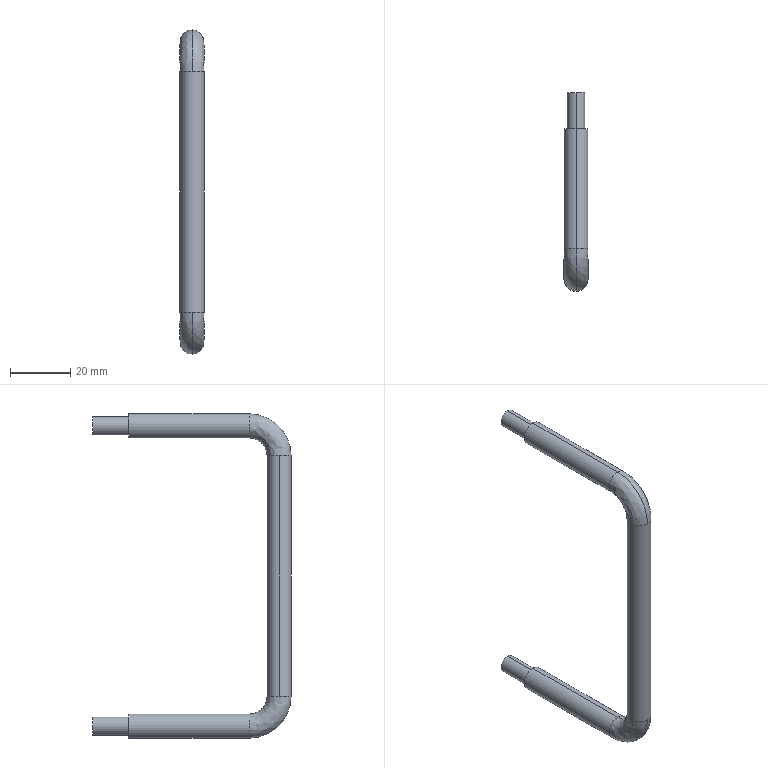Part | SolidWorks | features BaseBody 1 | 1 solid | 18 faces | box 8 x 66 x 108 mm | volume 10300 mm3 | cylinder 10 | spline 4 | plane 4 | commonest cylinder face diameters 8 x6 6 x4
STEP:
#1=CARTESIAN_POINT('',(331.946,-4131.973,2124.971));
#2=VERTEX_POINT('',#1);
#3=CARTESIAN_POINT('',(335.946,-4135.973,2124.971));
#4=VERTEX_POINT('',#3);
#5=CARTESIAN_POINT('',(331.946,-4135.973,2124.971));
#6=DIRECTION('',(0.,0.,-1.));
#7=DIRECTION('',(-1.,0.,0.));
#8=AXIS2_PLACEMENT_3D('',#5,#6,#7);
#9=CIRCLE('',#8,4.);
#10=EDGE_CURVE('',#2,#4,#9,.T.);
#11=ORIENTED_EDGE('',*,*,#10,.T.);
#12=CARTESIAN_POINT('',(335.946,-4135.973,2044.971));
#13=VERTEX_POINT('',#12);
#14=CARTESIAN_POINT('',(335.946,-4135.973,2044.971));
#15=DIRECTION('',(0.,0.,-1.));
#16=VECTOR('',#15,1000.);
#17=LINE('',#14,#16);
#18=EDGE_CURVE('',#4,#13,#17,.T.);
#19=ORIENTED_EDGE('',*,*,#18,.T.);
#20=CARTESIAN_POINT('',(331.946,-4131.973,2044.971));
#21=VERTEX_POINT('',#20);
#22=CARTESIAN_POINT('',(331.946,-4135.973,2044.971));
#23=DIRECTION('',(0.,0.,1.));
#24=DIRECTION('',(-1.,0.,0.));
#25=AXIS2_PLACEMENT_3D('',#22,#23,#24);
#26=CIRCLE('',#25,4.);
#27=EDGE_CURVE('',#13,#21,#26,.T.);
#28=ORIENTED_EDGE('',*,*,#27,.T.);
#29=CARTESIAN_POINT('',(327.946,-4135.973,2044.971));
#30=VERTEX_POINT('',#29);
#31=CARTESIAN_POINT('',(331.946,-4135.973,2044.971));
#32=DIRECTION('',(0.,0.,1.));
#33=DIRECTION('',(-1.,0.,0.));
#34=AXIS2_PLACEMENT_3D('',#31,#32,#33);
#35=CIRCLE('',#34,4.);
#36=EDGE_CURVE('',#21,#30,#35,.T.);
#37=ORIENTED_EDGE('',*,*,#36,.T.);
#38=CARTESIAN_POINT('',(327.946,-4135.973,2124.971));
#39=VERTEX_POINT('',#38);
#40=CARTESIAN_POINT('',(327.946,-4135.973,2044.971));
#41=DIRECTION('',(0.,0.,-1.));
#42=VECTOR('',#41,1000.);
#43=LINE('',#40,#42);
#44=EDGE_CURVE('',#39,#30,#43,.T.);
#45=ORIENTED_EDGE('',*,*,#44,.F.);
#46=CARTESIAN_POINT('',(331.946,-4135.973,2124.971));
#47=DIRECTION('',(0.,0.,-1.));
#48=DIRECTION('',(-1.,0.,0.));
#49=AXIS2_PLACEMENT_3D('',#46,#47,#48);
#50=CIRCLE('',#49,4.);
#51=EDGE_CURVE('',#39,#2,#50,.T.);
#52=ORIENTED_EDGE('',*,*,#51,.T.);
#53=EDGE_LOOP('',(#11,#19,#28,#37,#45,#52));
#54=FACE_OUTER_BOUND('',#53,.T.);
#55=CARTESIAN_POINT('',(331.946,-4135.973,2044.971));
#56=DIRECTION('',(0.,0.,-1.));
#57=DIRECTION('',(-1.,0.,0.));
#58=AXIS2_PLACEMENT_3D('',#55,#56,#57);
#59=CYLINDRICAL_SURFACE('',#58,4.);
#60=ADVANCED_FACE('',(#54),#59,.T.);
#61=ORIENTED_EDGE('',*,*,#36,.F.);
#62=CARTESIAN_POINT('',(331.946,-4125.973,2038.971));
#63=VERTEX_POINT('',#62);
#64=CARTESIAN_POINT('',(331.946,-4125.973,2044.971));
#65=DIRECTION('',(1.,0.,0.));
#66=DIRECTION('',(0.,0.,1.));
#67=AXIS2_PLACEMENT_3D('',#64,#65,#66);
#68=CIRCLE('',#67,6.);
#69=EDGE_CURVE('',#21,#63,#68,.T.);
#70=ORIENTED_EDGE('',*,*,#69,.T.);
#71=CARTESIAN_POINT('',(331.946,-4125.973,2030.971));
#72=VERTEX_POINT('',#71);
#73=CARTESIAN_POINT('',(331.946,-4125.973,2034.971));
#74=DIRECTION('',(0.,-1.,0.));
#75=DIRECTION('',(0.,0.,-1.));
#76=AXIS2_PLACEMENT_3D('',#73,#74,#75);
#77=CIRCLE('',#76,4.);
#78=EDGE_CURVE('',#63,#72,#77,.T.);
#79=ORIENTED_EDGE('',*,*,#78,.T.);
#80=CARTESIAN_POINT('',(331.946,-4139.973,2044.971));
#81=VERTEX_POINT('',#80);
#82=CARTESIAN_POINT('',(331.946,-4125.973,2044.971));
#83=DIRECTION('',(1.,0.,0.));
#84=DIRECTION('',(0.,0.,1.));
#85=AXIS2_PLACEMENT_3D('',#82,#83,#84);
#86=CIRCLE('',#85,14.);
#87=EDGE_CURVE('',#81,#72,#86,.T.);
#88=ORIENTED_EDGE('',*,*,#87,.F.);
#89=CARTESIAN_POINT('',(331.946,-4135.973,2044.971));
#90=DIRECTION('',(0.,0.,1.));
#91=DIRECTION('',(-1.,0.,0.));
#92=AXIS2_PLACEMENT_3D('',#89,#90,#91);
#93=CIRCLE('',#92,4.);
#94=EDGE_CURVE('',#30,#81,#93,.T.);
#95=ORIENTED_EDGE('',*,*,#94,.F.);
#96=EDGE_LOOP('',(#61,#70,#79,#88,#95));
#97=FACE_OUTER_BOUND('',#96,.T.);
#98=CARTESIAN_POINT('',(331.946,-4139.973,2044.971));
#99=CARTESIAN_POINT('',(331.946,-4139.973,2036.77));
#100=CARTESIAN_POINT('',(331.946,-4134.174,2030.971));
#101=CARTESIAN_POINT('',(331.946,-4125.973,2030.971));
#102=CARTESIAN_POINT('',(323.946,-4139.973,2044.971));
#103=CARTESIAN_POINT('',(323.946,-4139.973,2036.77));
#104=CARTESIAN_POINT('',(323.946,-4134.174,2030.971));
#105=CARTESIAN_POINT('',(323.946,-4125.973,2030.971));
#106=CARTESIAN_POINT('',(323.946,-4131.973,2044.971));
#107=CARTESIAN_POINT('',(323.946,-4131.973,2041.457));
#108=CARTESIAN_POINT('',(323.946,-4129.488,2038.971));
#109=CARTESIAN_POINT('',(323.946,-4125.973,2038.971));
#110=CARTESIAN_POINT('',(331.946,-4131.973,2044.971));
#111=CARTESIAN_POINT('',(331.946,-4131.973,2041.457));
#112=CARTESIAN_POINT('',(331.946,-4129.488,2038.971));
#113=CARTESIAN_POINT('',(331.946,-4125.973,2038.971));
#114=(BOUNDED_SURFACE()B_SPLINE_SURFACE(3,3,((#98,#99,#100,#101),(#102,#103,#104,#105),(#106,#107,#108,#109),(#110,#111,#112,#113)),.UNSPECIFIED.,.F.,.F.,.F.)B_SPLINE_SURFACE_WITH_KNOTS((4,4),(4,4),(0.,1.),(0.,1.),.UNSPECIFIED.)GEOMETRIC_REPRESENTATION_ITEM()RATIONAL_B_SPLINE_SURFACE(((1.,0.8047,0.8047,1.),(0.3333,0.2682,0.2682,0.3333),(0.3333,0.2682,0.2682,0.3333),(1.,0.8047,0.8047,1.)))REPRESENTATION_ITEM('')SURFACE());
#115=ADVANCED_FACE('',(#97),#114,.T.);
#116=CARTESIAN_POINT('',(331.946,-4125.973,2138.971));
#117=VERTEX_POINT('',#116);
#118=CARTESIAN_POINT('',(331.946,-4125.973,2130.971));
#119=VERTEX_POINT('',#118);
#120=CARTESIAN_POINT('',(331.946,-4125.973,2134.971));
#121=DIRECTION('',(0.,-1.,0.));
#122=DIRECTION('',(0.,0.,1.));
#123=AXIS2_PLACEMENT_3D('',#120,#121,#122);
#124=CIRCLE('',#123,4.);
#125=EDGE_CURVE('',#117,#119,#124,.T.);
#126=ORIENTED_EDGE('',*,*,#125,.T.);
#127=CARTESIAN_POINT('',(331.946,-4125.973,2124.971));
#128=DIRECTION('',(1.,0.,0.));
#129=DIRECTION('',(0.,0.,1.));
#130=AXIS2_PLACEMENT_3D('',#127,#128,#129);
#131=CIRCLE('',#130,6.);
#132=EDGE_CURVE('',#119,#2,#131,.T.);
#133=ORIENTED_EDGE('',*,*,#132,.T.);
#134=ORIENTED_EDGE('',*,*,#51,.F.);
#135=CARTESIAN_POINT('',(331.946,-4139.973,2124.971));
#136=VERTEX_POINT('',#135);
#137=CARTESIAN_POINT('',(331.946,-4135.973,2124.971));
#138=DIRECTION('',(0.,0.,-1.));
#139=DIRECTION('',(-1.,0.,0.));
#140=AXIS2_PLACEMENT_3D('',#137,#138,#139);
#141=CIRCLE('',#140,4.);
#142=EDGE_CURVE('',#136,#39,#141,.T.);
#143=ORIENTED_EDGE('',*,*,#142,.F.);
#144=CARTESIAN_POINT('',(331.946,-4125.973,2124.971));
#145=DIRECTION('',(1.,0.,0.));
#146=DIRECTION('',(0.,0.,1.));
#147=AXIS2_PLACEMENT_3D('',#144,#145,#146);
#148=CIRCLE('',#147,14.);
#149=EDGE_CURVE('',#117,#136,#148,.T.);
#150=ORIENTED_EDGE('',*,*,#149,.F.);
#151=EDGE_LOOP('',(#126,#133,#134,#143,#150));
#152=FACE_OUTER_BOUND('',#151,.T.);
#153=CARTESIAN_POINT('',(331.946,-4125.973,2138.971));
#154=CARTESIAN_POINT('',(331.946,-4134.174,2138.971));
#155=CARTESIAN_POINT('',(331.946,-4139.973,2133.172));
#156=CARTESIAN_POINT('',(331.946,-4139.973,2124.971));
#157=CARTESIAN_POINT('',(323.946,-4125.973,2138.971));
#158=CARTESIAN_POINT('',(323.946,-4134.174,2138.971));
#159=CARTESIAN_POINT('',(323.946,-4139.973,2133.172));
#160=CARTESIAN_POINT('',(323.946,-4139.973,2124.971));
#161=CARTESIAN_POINT('',(323.946,-4125.973,2130.971));
#162=CARTESIAN_POINT('',(323.946,-4129.488,2130.971));
#163=CARTESIAN_POINT('',(323.946,-4131.973,2128.486));
#164=CARTESIAN_POINT('',(323.946,-4131.973,2124.971));
#165=CARTESIAN_POINT('',(331.946,-4125.973,2130.971));
#166=CARTESIAN_POINT('',(331.946,-4129.488,2130.971));
#167=CARTESIAN_POINT('',(331.946,-4131.973,2128.486));
#168=CARTESIAN_POINT('',(331.946,-4131.973,2124.971));
#169=(BOUNDED_SURFACE()B_SPLINE_SURFACE(3,3,((#153,#154,#155,#156),(#157,#158,#159,#160),(#161,#162,#163,#164),(#165,#166,#167,#168)),.UNSPECIFIED.,.F.,.F.,.F.)B_SPLINE_SURFACE_WITH_KNOTS((4,4),(4,4),(0.,1.),(0.,1.),.UNSPECIFIED.)GEOMETRIC_REPRESENTATION_ITEM()RATIONAL_B_SPLINE_SURFACE(((1.,0.8047,0.8047,1.),(0.3333,0.2682,0.2682,0.3333),(0.3333,0.2682,0.2682,0.3333),(1.,0.8047,0.8047,1.)))REPRESENTATION_ITEM('')SURFACE());
#170=ADVANCED_FACE('',(#152),#169,.T.);
#171=CARTESIAN_POINT('',(331.946,-4125.973,2034.971));
#172=DIRECTION('',(0.,-1.,0.));
#173=DIRECTION('',(0.,0.,-1.));
#174=AXIS2_PLACEMENT_3D('',#171,#172,#173);
#175=CIRCLE('',#174,4.);
#176=EDGE_CURVE('',#72,#63,#175,.T.);
#177=ORIENTED_EDGE('',*,*,#176,.F.);
#178=CARTESIAN_POINT('',(331.946,-4085.973,2030.971));
#179=VERTEX_POINT('',#178);
#180=CARTESIAN_POINT('',(331.946,-4085.973,2030.971));
#181=DIRECTION('',(0.,1.,0.));
#182=VECTOR('',#181,1000.);
#183=LINE('',#180,#182);
#184=EDGE_CURVE('',#72,#179,#183,.T.);
#185=ORIENTED_EDGE('',*,*,#184,.T.);
#186=CARTESIAN_POINT('',(331.946,-4085.973,2038.971));
#187=VERTEX_POINT('',#186);
#188=CARTESIAN_POINT('',(331.946,-4085.973,2034.971));
#189=DIRECTION('',(0.,-1.,0.));
#190=DIRECTION('',(0.,0.,1.));
#191=AXIS2_PLACEMENT_3D('',#188,#189,#190);
#192=CIRCLE('',#191,4.);
#193=EDGE_CURVE('',#179,#187,#192,.T.);
#194=ORIENTED_EDGE('',*,*,#193,.T.);
#195=CARTESIAN_POINT('',(331.946,-4085.973,2038.971));
#196=DIRECTION('',(0.,1.,0.));
#197=VECTOR('',#196,1000.);
#198=LINE('',#195,#197);
#199=EDGE_CURVE('',#63,#187,#198,.T.);
#200=ORIENTED_EDGE('',*,*,#199,.F.);
#201=EDGE_LOOP('',(#177,#185,#194,#200));
#202=FACE_OUTER_BOUND('',#201,.T.);
#203=CARTESIAN_POINT('',(331.946,-4085.973,2034.971));
#204=DIRECTION('',(0.,1.,0.));
#205=DIRECTION('',(0.,0.,1.));
#206=AXIS2_PLACEMENT_3D('',#203,#204,#205);
#207=CYLINDRICAL_SURFACE('',#206,4.);
#208=ADVANCED_FACE('',(#202),#207,.T.);
#209=CARTESIAN_POINT('',(331.946,-4085.973,2130.971));
#210=VERTEX_POINT('',#209);
#211=CARTESIAN_POINT('',(331.946,-4085.973,2138.971));
#212=VERTEX_POINT('',#211);
#213=CARTESIAN_POINT('',(331.946,-4085.973,2134.971));
#214=DIRECTION('',(0.,-1.,0.));
#215=DIRECTION('',(0.,0.,-1.));
#216=AXIS2_PLACEMENT_3D('',#213,#214,#215);
#217=CIRCLE('',#216,4.);
#218=EDGE_CURVE('',#210,#212,#217,.T.);
#219=ORIENTED_EDGE('',*,*,#218,.T.);
#220=CARTESIAN_POINT('',(331.946,-4125.973,2138.971));
#221=DIRECTION('',(0.,-1.,0.));
#222=VECTOR('',#221,1000.);
#223=LINE('',#220,#222);
#224=EDGE_CURVE('',#212,#117,#223,.T.);
#225=ORIENTED_EDGE('',*,*,#224,.T.);
#226=CARTESIAN_POINT('',(331.946,-4125.973,2134.971));
#227=DIRECTION('',(0.,-1.,0.));
#228=DIRECTION('',(0.,0.,1.));
#229=AXIS2_PLACEMENT_3D('',#226,#227,#228);
#230=CIRCLE('',#229,4.);
#231=EDGE_CURVE('',#119,#117,#230,.T.);
#232=ORIENTED_EDGE('',*,*,#231,.F.);
#233=CARTESIAN_POINT('',(331.946,-4125.973,2130.971));
#234=DIRECTION('',(0.,-1.,0.));
#235=VECTOR('',#234,1000.);
#236=LINE('',#233,#235);
#237=EDGE_CURVE('',#210,#119,#236,.T.);
#238=ORIENTED_EDGE('',*,*,#237,.F.);
#239=EDGE_LOOP('',(#219,#225,#232,#238));
#240=FACE_OUTER_BOUND('',#239,.T.);
#241=CARTESIAN_POINT('',(331.946,-4125.973,2134.971));
#242=DIRECTION('',(0.,-1.,0.));
#243=DIRECTION('',(0.,0.,-1.));
#244=AXIS2_PLACEMENT_3D('',#241,#242,#243);
#245=CYLINDRICAL_SURFACE('',#244,4.);
#246=ADVANCED_FACE('',(#240),#245,.T.);
#247=CARTESIAN_POINT('',(331.946,-4073.973,2031.971));
#248=VERTEX_POINT('',#247);
#249=CARTESIAN_POINT('',(331.946,-4073.973,2037.971));
#250=VERTEX_POINT('',#249);
#251=CARTESIAN_POINT('',(331.946,-4073.973,2034.971));
#252=DIRECTION('',(0.,-1.,0.));
#253=DIRECTION('',(0.,0.,-1.));
#254=AXIS2_PLACEMENT_3D('',#251,#252,#253);
#255=CIRCLE('',#254,3.);
#256=EDGE_CURVE('',#248,#250,#255,.T.);
#257=ORIENTED_EDGE('',*,*,#256,.T.);
#258=CARTESIAN_POINT('',(331.946,-4085.973,2037.971));
#259=VERTEX_POINT('',#258);
#260=CARTESIAN_POINT('',(331.946,-4079.973,2037.971));
#261=DIRECTION('',(0.,-1.,0.));
#262=VECTOR('',#261,1000.);
#263=LINE('',#260,#262);
#264=EDGE_CURVE('',#250,#259,#263,.T.);
#265=ORIENTED_EDGE('',*,*,#264,.T.);
#266=CARTESIAN_POINT('',(331.946,-4085.973,2031.971));
#267=VERTEX_POINT('',#266);
#268=CARTESIAN_POINT('',(331.946,-4085.973,2034.971));
#269=DIRECTION('',(0.,-1.,0.));
#270=DIRECTION('',(0.,0.,-1.));
#271=AXIS2_PLACEMENT_3D('',#268,#269,#270);
#272=CIRCLE('',#271,3.);
#273=EDGE_CURVE('',#267,#259,#272,.T.);
#274=ORIENTED_EDGE('',*,*,#273,.F.);
#275=CARTESIAN_POINT('',(331.946,-4079.973,2031.971));
#276=DIRECTION('',(0.,-1.,0.));
#277=VECTOR('',#276,1000.);
#278=LINE('',#275,#277);
#279=EDGE_CURVE('',#248,#267,#278,.T.);
#280=ORIENTED_EDGE('',*,*,#279,.F.);
#281=EDGE_LOOP('',(#257,#265,#274,#280));
#282=FACE_OUTER_BOUND('',#281,.T.);
#283=CARTESIAN_POINT('',(331.946,-4079.973,2034.971));
#284=DIRECTION('',(0.,-1.,0.));
#285=DIRECTION('',(0.,0.,-1.));
#286=AXIS2_PLACEMENT_3D('',#283,#284,#285);
#287=CYLINDRICAL_SURFACE('',#286,3.);
#288=ADVANCED_FACE('',(#282),#287,.T.);
#289=CARTESIAN_POINT('',(331.946,-4085.973,2137.971));
#290=VERTEX_POINT('',#289);
#291=CARTESIAN_POINT('',(331.946,-4085.973,2131.971));
#292=VERTEX_POINT('',#291);
#293=CARTESIAN_POINT('',(331.946,-4085.973,2134.971));
#294=DIRECTION('',(0.,1.,0.));
#295=DIRECTION('',(0.,0.,1.));
#296=AXIS2_PLACEMENT_3D('',#293,#294,#295);
#297=CIRCLE('',#296,3.);
#298=EDGE_CURVE('',#290,#292,#297,.T.);
#299=ORIENTED_EDGE('',*,*,#298,.T.);
#300=CARTESIAN_POINT('',(331.946,-4073.973,2131.971));
#301=VERTEX_POINT('',#300);
#302=CARTESIAN_POINT('',(331.946,-4079.973,2131.971));
#303=DIRECTION('',(0.,1.,0.));
#304=VECTOR('',#303,1000.);
#305=LINE('',#302,#304);
#306=EDGE_CURVE('',#292,#301,#305,.T.);
#307=ORIENTED_EDGE('',*,*,#306,.T.);
#308=CARTESIAN_POINT('',(331.946,-4073.973,2137.971));
#309=VERTEX_POINT('',#308);
#310=CARTESIAN_POINT('',(331.946,-4073.973,2134.971));
#311=DIRECTION('',(0.,-1.,0.));
#312=DIRECTION('',(0.,0.,1.));
#313=AXIS2_PLACEMENT_3D('',#310,#311,#312);
#314=CIRCLE('',#313,3.);
#315=EDGE_CURVE('',#301,#309,#314,.T.);
#316=ORIENTED_EDGE('',*,*,#315,.T.);
#317=CARTESIAN_POINT('',(331.946,-4079.973,2137.971));
#318=DIRECTION('',(0.,1.,0.));
#319=VECTOR('',#318,1000.);
#320=LINE('',#317,#319);
#321=EDGE_CURVE('',#290,#309,#320,.T.);
#322=ORIENTED_EDGE('',*,*,#321,.F.);
#323=EDGE_LOOP('',(#299,#307,#316,#322));
#324=FACE_OUTER_BOUND('',#323,.T.);
#325=CARTESIAN_POINT('',(331.946,-4079.973,2134.971));
#326=DIRECTION('',(0.,1.,0.));
#327=DIRECTION('',(0.,0.,1.));
#328=AXIS2_PLACEMENT_3D('',#325,#326,#327);
#329=CYLINDRICAL_SURFACE('',#328,3.);
#330=ADVANCED_FACE('',(#324),#329,.T.);
#331=ORIENTED_EDGE('',*,*,#18,.F.);
#332=CARTESIAN_POINT('',(331.946,-4135.973,2124.971));
#333=DIRECTION('',(0.,0.,-1.));
#334=DIRECTION('',(-1.,0.,0.));
#335=AXIS2_PLACEMENT_3D('',#332,#333,#334);
#336=CIRCLE('',#335,4.);
#337=EDGE_CURVE('',#4,#136,#336,.T.);
#338=ORIENTED_EDGE('',*,*,#337,.T.);
#339=ORIENTED_EDGE('',*,*,#142,.T.);
#340=ORIENTED_EDGE('',*,*,#44,.T.);
#341=ORIENTED_EDGE('',*,*,#94,.T.);
#342=CARTESIAN_POINT('',(331.946,-4135.973,2044.971));
#343=DIRECTION('',(0.,0.,1.));
#344=DIRECTION('',(-1.,0.,0.));
#345=AXIS2_PLACEMENT_3D('',#342,#343,#344);
#346=CIRCLE('',#345,4.);
#347=EDGE_CURVE('',#81,#13,#346,.T.);
#348=ORIENTED_EDGE('',*,*,#347,.T.);
#349=EDGE_LOOP('',(#331,#338,#339,#340,#341,#348));
#350=FACE_OUTER_BOUND('',#349,.T.);
#351=CARTESIAN_POINT('',(331.946,-4135.973,2044.971));
#352=DIRECTION('',(0.,0.,-1.));
#353=DIRECTION('',(-1.,0.,0.));
#354=AXIS2_PLACEMENT_3D('',#351,#352,#353);
#355=CYLINDRICAL_SURFACE('',#354,4.);
#356=ADVANCED_FACE('',(#350),#355,.T.);
#357=ORIENTED_EDGE('',*,*,#69,.F.);
#358=ORIENTED_EDGE('',*,*,#27,.F.);
#359=ORIENTED_EDGE('',*,*,#347,.F.);
#360=ORIENTED_EDGE('',*,*,#87,.T.);
#361=ORIENTED_EDGE('',*,*,#176,.T.);
#362=EDGE_LOOP('',(#357,#358,#359,#360,#361));
#363=FACE_OUTER_BOUND('',#362,.T.);
#364=CARTESIAN_POINT('',(331.946,-4131.973,2044.971));
#365=CARTESIAN_POINT('',(331.946,-4131.973,2041.457));
#366=CARTESIAN_POINT('',(331.946,-4129.488,2038.971));
#367=CARTESIAN_POINT('',(331.946,-4125.973,2038.971));
#368=CARTESIAN_POINT('',(339.946,-4131.973,2044.971));
#369=CARTESIAN_POINT('',(339.946,-4131.973,2041.457));
#370=CARTESIAN_POINT('',(339.946,-4129.488,2038.971));
#371=CARTESIAN_POINT('',(339.946,-4125.973,2038.971));
#372=CARTESIAN_POINT('',(339.946,-4139.973,2044.971));
#373=CARTESIAN_POINT('',(339.946,-4139.973,2036.77));
#374=CARTESIAN_POINT('',(339.946,-4134.174,2030.971));
#375=CARTESIAN_POINT('',(339.946,-4125.973,2030.971));
#376=CARTESIAN_POINT('',(331.946,-4139.973,2044.971));
#377=CARTESIAN_POINT('',(331.946,-4139.973,2036.77));
#378=CARTESIAN_POINT('',(331.946,-4134.174,2030.971));
#379=CARTESIAN_POINT('',(331.946,-4125.973,2030.971));
#380=(BOUNDED_SURFACE()B_SPLINE_SURFACE(3,3,((#364,#365,#366,#367),(#368,#369,#370,#371),(#372,#373,#374,#375),(#376,#377,#378,#379)),.UNSPECIFIED.,.F.,.F.,.F.)B_SPLINE_SURFACE_WITH_KNOTS((4,4),(4,4),(0.,1.),(0.,1.),.UNSPECIFIED.)GEOMETRIC_REPRESENTATION_ITEM()RATIONAL_B_SPLINE_SURFACE(((1.,0.8047,0.8047,1.),(0.3333,0.2682,0.2682,0.3333),(0.3333,0.2682,0.2682,0.3333),(1.,0.8047,0.8047,1.)))REPRESENTATION_ITEM('')SURFACE());
#381=ADVANCED_FACE('',(#363),#380,.T.);
#382=ORIENTED_EDGE('',*,*,#132,.F.);
#383=ORIENTED_EDGE('',*,*,#231,.T.);
#384=ORIENTED_EDGE('',*,*,#149,.T.);
#385=ORIENTED_EDGE('',*,*,#337,.F.);
#386=ORIENTED_EDGE('',*,*,#10,.F.);
#387=EDGE_LOOP('',(#382,#383,#384,#385,#386));
#388=FACE_OUTER_BOUND('',#387,.T.);
#389=CARTESIAN_POINT('',(331.946,-4125.973,2130.971));
#390=CARTESIAN_POINT('',(331.946,-4129.488,2130.971));
#391=CARTESIAN_POINT('',(331.946,-4131.973,2128.486));
#392=CARTESIAN_POINT('',(331.946,-4131.973,2124.971));
#393=CARTESIAN_POINT('',(339.946,-4125.973,2130.971));
#394=CARTESIAN_POINT('',(339.946,-4129.488,2130.971));
#395=CARTESIAN_POINT('',(339.946,-4131.973,2128.486));
#396=CARTESIAN_POINT('',(339.946,-4131.973,2124.971));
#397=CARTESIAN_POINT('',(339.946,-4125.973,2138.971));
#398=CARTESIAN_POINT('',(339.946,-4134.174,2138.971));
#399=CARTESIAN_POINT('',(339.946,-4139.973,2133.172));
#400=CARTESIAN_POINT('',(339.946,-4139.973,2124.971));
#401=CARTESIAN_POINT('',(331.946,-4125.973,2138.971));
#402=CARTESIAN_POINT('',(331.946,-4134.174,2138.971));
#403=CARTESIAN_POINT('',(331.946,-4139.973,2133.172));
#404=CARTESIAN_POINT('',(331.946,-4139.973,2124.971));
#405=(BOUNDED_SURFACE()B_SPLINE_SURFACE(3,3,((#389,#390,#391,#392),(#393,#394,#395,#396),(#397,#398,#399,#400),(#401,#402,#403,#404)),.UNSPECIFIED.,.F.,.F.,.F.)B_SPLINE_SURFACE_WITH_KNOTS((4,4),(4,4),(0.,1.),(0.,1.),.UNSPECIFIED.)GEOMETRIC_REPRESENTATION_ITEM()RATIONAL_B_SPLINE_SURFACE(((1.,0.8047,0.8047,1.),(0.3333,0.2682,0.2682,0.3333),(0.3333,0.2682,0.2682,0.3333),(1.,0.8047,0.8047,1.)))REPRESENTATION_ITEM('')SURFACE());
#406=ADVANCED_FACE('',(#388),#405,.T.);
#407=ORIENTED_EDGE('',*,*,#184,.F.);
#408=ORIENTED_EDGE('',*,*,#78,.F.);
#409=ORIENTED_EDGE('',*,*,#199,.T.);
#410=CARTESIAN_POINT('',(331.946,-4085.973,2034.971));
#411=DIRECTION('',(0.,-1.,0.));
#412=DIRECTION('',(0.,0.,1.));
#413=AXIS2_PLACEMENT_3D('',#410,#411,#412);
#414=CIRCLE('',#413,4.);
#415=EDGE_CURVE('',#187,#179,#414,.T.);
#416=ORIENTED_EDGE('',*,*,#415,.T.);
#417=EDGE_LOOP('',(#407,#408,#409,#416));
#418=FACE_OUTER_BOUND('',#417,.T.);
#419=CARTESIAN_POINT('',(331.946,-4085.973,2034.971));
#420=DIRECTION('',(0.,1.,0.));
#421=DIRECTION('',(0.,0.,1.));
#422=AXIS2_PLACEMENT_3D('',#419,#420,#421);
#423=CYLINDRICAL_SURFACE('',#422,4.);
#424=ADVANCED_FACE('',(#418),#423,.T.);
#425=ORIENTED_EDGE('',*,*,#224,.F.);
#426=CARTESIAN_POINT('',(331.946,-4085.973,2134.971));
#427=DIRECTION('',(0.,-1.,0.));
#428=DIRECTION('',(0.,0.,-1.));
#429=AXIS2_PLACEMENT_3D('',#426,#427,#428);
#430=CIRCLE('',#429,4.);
#431=EDGE_CURVE('',#212,#210,#430,.T.);
#432=ORIENTED_EDGE('',*,*,#431,.T.);
#433=ORIENTED_EDGE('',*,*,#237,.T.);
#434=ORIENTED_EDGE('',*,*,#125,.F.);
#435=EDGE_LOOP('',(#425,#432,#433,#434));
#436=FACE_OUTER_BOUND('',#435,.T.);
#437=CARTESIAN_POINT('',(331.946,-4125.973,2134.971));
#438=DIRECTION('',(0.,-1.,0.));
#439=DIRECTION('',(0.,0.,-1.));
#440=AXIS2_PLACEMENT_3D('',#437,#438,#439);
#441=CYLINDRICAL_SURFACE('',#440,4.);
#442=ADVANCED_FACE('',(#436),#441,.T.);
#443=ORIENTED_EDGE('',*,*,#273,.T.);
#444=CARTESIAN_POINT('',(331.946,-4085.973,2034.971));
#445=DIRECTION('',(0.,-1.,0.));
#446=DIRECTION('',(0.,0.,-1.));
#447=AXIS2_PLACEMENT_3D('',#444,#445,#446);
#448=CIRCLE('',#447,3.);
#449=EDGE_CURVE('',#259,#267,#448,.T.);
#450=ORIENTED_EDGE('',*,*,#449,.T.);
#451=EDGE_LOOP('',(#443,#450));
#452=FACE_BOUND('',#451,.T.);
#453=ORIENTED_EDGE('',*,*,#415,.F.);
#454=ORIENTED_EDGE('',*,*,#193,.F.);
#455=EDGE_LOOP('',(#453,#454));
#456=FACE_OUTER_BOUND('',#455,.T.);
#457=CARTESIAN_POINT('',(331.946,-4085.973,2034.971));
#458=DIRECTION('',(0.,1.,0.));
#459=DIRECTION('',(0.,0.,1.));
#460=AXIS2_PLACEMENT_3D('',#457,#458,#459);
#461=PLANE('',#460);
#462=ADVANCED_FACE('',(#452,#456),#461,.T.);
#463=ORIENTED_EDGE('',*,*,#298,.F.);
#464=CARTESIAN_POINT('',(331.946,-4085.973,2134.971));
#465=DIRECTION('',(0.,1.,0.));
#466=DIRECTION('',(0.,0.,1.));
#467=AXIS2_PLACEMENT_3D('',#464,#465,#466);
#468=CIRCLE('',#467,3.);
#469=EDGE_CURVE('',#292,#290,#468,.T.);
#470=ORIENTED_EDGE('',*,*,#469,.F.);
#471=EDGE_LOOP('',(#463,#470));
#472=FACE_BOUND('',#471,.T.);
#473=ORIENTED_EDGE('',*,*,#218,.F.);
#474=ORIENTED_EDGE('',*,*,#431,.F.);
#475=EDGE_LOOP('',(#473,#474));
#476=FACE_OUTER_BOUND('',#475,.T.);
#477=CARTESIAN_POINT('',(331.946,-4085.973,2134.971));
#478=DIRECTION('',(0.,-1.,0.));
#479=DIRECTION('',(0.,0.,-1.));
#480=AXIS2_PLACEMENT_3D('',#477,#478,#479);
#481=PLANE('',#480);
#482=ADVANCED_FACE('',(#472,#476),#481,.F.);
#483=ORIENTED_EDGE('',*,*,#264,.F.);
#484=CARTESIAN_POINT('',(331.946,-4073.973,2034.971));
#485=DIRECTION('',(0.,-1.,0.));
#486=DIRECTION('',(0.,0.,-1.));
#487=AXIS2_PLACEMENT_3D('',#484,#485,#486);
#488=CIRCLE('',#487,3.);
#489=EDGE_CURVE('',#250,#248,#488,.T.);
#490=ORIENTED_EDGE('',*,*,#489,.T.);
#491=ORIENTED_EDGE('',*,*,#279,.T.);
#492=ORIENTED_EDGE('',*,*,#449,.F.);
#493=EDGE_LOOP('',(#483,#490,#491,#492));
#494=FACE_OUTER_BOUND('',#493,.T.);
#495=CARTESIAN_POINT('',(331.946,-4079.973,2034.971));
#496=DIRECTION('',(0.,-1.,0.));
#497=DIRECTION('',(0.,0.,-1.));
#498=AXIS2_PLACEMENT_3D('',#495,#496,#497);
#499=CYLINDRICAL_SURFACE('',#498,3.);
#500=ADVANCED_FACE('',(#494),#499,.T.);
#501=ORIENTED_EDGE('',*,*,#306,.F.);
#502=ORIENTED_EDGE('',*,*,#469,.T.);
#503=ORIENTED_EDGE('',*,*,#321,.T.);
#504=CARTESIAN_POINT('',(331.946,-4073.973,2134.971));
#505=DIRECTION('',(0.,-1.,0.));
#506=DIRECTION('',(0.,0.,1.));
#507=AXIS2_PLACEMENT_3D('',#504,#505,#506);
#508=CIRCLE('',#507,3.);
#509=EDGE_CURVE('',#309,#301,#508,.T.);
#510=ORIENTED_EDGE('',*,*,#509,.T.);
#511=EDGE_LOOP('',(#501,#502,#503,#510));
#512=FACE_OUTER_BOUND('',#511,.T.);
#513=CARTESIAN_POINT('',(331.946,-4079.973,2134.971));
#514=DIRECTION('',(0.,1.,0.));
#515=DIRECTION('',(0.,0.,1.));
#516=AXIS2_PLACEMENT_3D('',#513,#514,#515);
#517=CYLINDRICAL_SURFACE('',#516,3.);
#518=ADVANCED_FACE('',(#512),#517,.T.);
#519=ORIENTED_EDGE('',*,*,#256,.F.);
#520=ORIENTED_EDGE('',*,*,#489,.F.);
#521=EDGE_LOOP('',(#519,#520));
#522=FACE_OUTER_BOUND('',#521,.T.);
#523=CARTESIAN_POINT('',(331.946,-4073.973,2034.971));
#524=DIRECTION('',(0.,1.,0.));
#525=DIRECTION('',(0.,0.,1.));
#526=AXIS2_PLACEMENT_3D('',#523,#524,#525);
#527=PLANE('',#526);
#528=ADVANCED_FACE('',(#522),#527,.T.);
#529=ORIENTED_EDGE('',*,*,#509,.F.);
#530=ORIENTED_EDGE('',*,*,#315,.F.);
#531=EDGE_LOOP('',(#529,#530));
#532=FACE_OUTER_BOUND('',#531,.T.);
#533=CARTESIAN_POINT('',(331.946,-4073.973,2134.971));
#534=DIRECTION('',(0.,1.,0.));
#535=DIRECTION('',(0.,0.,1.));
#536=AXIS2_PLACEMENT_3D('',#533,#534,#535);
#537=PLANE('',#536);
#538=ADVANCED_FACE('',(#532),#537,.T.);
#539=CLOSED_SHELL('',(#60,#115,#170,#208,#246,#288,#330,#356,#381,#406,#424,#442,#462,#482,#500,#518,#528,#538));
#540=MANIFOLD_SOLID_BREP('',#539);
#541=CARTESIAN_POINT('',(0.,0.,0.));
#542=DIRECTION('',(0.,0.,1.));
#543=DIRECTION('',(1.,0.,0.));
#544=AXIS2_PLACEMENT_3D('',#541,#542,#543);
#545=(LENGTH_UNIT()NAMED_UNIT(*)SI_UNIT(.MILLI.,.METRE.));
#546=UNCERTAINTY_MEASURE_WITH_UNIT(LENGTH_MEASURE(0.00001),#545,'','');
#547=(NAMED_UNIT(*)PLANE_ANGLE_UNIT()SI_UNIT($,.RADIAN.));
#548=(NAMED_UNIT(*)SI_UNIT($,.STERADIAN.)SOLID_ANGLE_UNIT());
#549=(GEOMETRIC_REPRESENTATION_CONTEXT(3)GLOBAL_UNCERTAINTY_ASSIGNED_CONTEXT((#546))GLOBAL_UNIT_ASSIGNED_CONTEXT((#545,#547,#548))REPRESENTATION_CONTEXT('',''));
#550=ADVANCED_BREP_SHAPE_REPRESENTATION('',(#540,#544),#549);